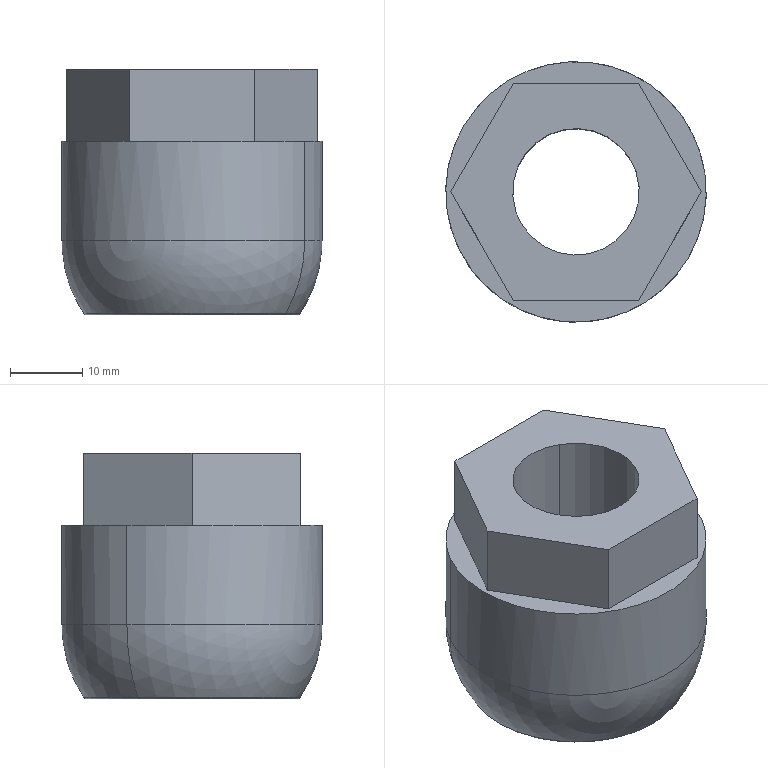NC program | NX | posted with a generic post | part box 36 x 36 x 34 mm
Lines 1 to 932 of 2807:
N10 G17 G21 G94 G90
(ZLEVEL_PROFILE , TOOL : D6C)
N12 T06 M6
N14 G54
N16 G17 G0 G90 X-11.017 Y-16.863 S4000 M3
N18 G43 Z30. H6
N20 Z1.5
N22 G94 G1 X-11.144 Y-16.717 Z1.49 F1800.
N24 X-20.05 Y-1.292 Z0.556
N26 X-20.266 Y-0.662 Z0.521
N28 X-20.34 Y0. Z0.487
N30 X-20.266 Y0.662 Z0.452
N32 X-20.05 Y1.292 Z0.417
N34 X-15.597 Y9.005 Z-0.05
N36 X-11.267 Y16.505
N38 G2 X-8.66 Y18.01 R3.01
N40 G1 X8.66
N42 G2 X11.267 Y16.505 R3.01
N44 G1 X19.927 Y1.505
N46 G2 X19.927 Y-1.505 R3.01
N48 G1 X11.267 Y-16.505
N50 G2 X8.66 Y-18.01 R3.01
N52 G1 X-8.66
N54 G2 X-11.267 Y-16.505 R3.01
N56 G1 X-19.927 Y-1.505
N58 G2 X-19.927 Y1.505 R3.01
N60 G1 X-15.597 Y9.005
N62 X-14.164 Y11.486 Z-0.1
N64 X-11.267 Y16.505
N66 G2 X-8.66 Y18.01 R3.01
N68 G1 X8.66
N70 G2 X11.267 Y16.505 R3.01
N72 G1 X19.927 Y1.505
N74 G2 X19.927 Y-1.505 R3.01
N76 G1 X11.267 Y-16.505
N78 G2 X8.66 Y-18.01 R3.01
N80 G1 X-8.66
N82 G2 X-11.267 Y-16.505 R3.01
N84 G1 X-19.927 Y-1.505
N86 G2 X-19.927 Y1.505 R3.01
N88 G1 X-15.597 Y9.005
N90 X-14.164 Y11.486 Z-0.15
N92 X-11.267 Y16.505
N94 G2 X-8.66 Y18.01 R3.01
N96 G1 X8.66
N98 G2 X11.267 Y16.505 R3.01
N100 G1 X19.927 Y1.505
N102 G2 X19.927 Y-1.505 R3.01
N104 G1 X11.267 Y-16.505
N106 G2 X8.66 Y-18.01 R3.01
N108 G1 X-8.66
N110 G2 X-11.267 Y-16.505 R3.01
N112 G1 X-19.927 Y-1.505
N114 G2 X-19.927 Y1.505 R3.01
N116 G1 X-15.597 Y9.005
N118 X-14.164 Y11.486 Z-0.2
N120 X-11.267 Y16.505
N122 G2 X-8.66 Y18.01 R3.01
N124 G1 X8.66
N126 G2 X11.267 Y16.505 R3.01
N128 G1 X19.927 Y1.505
N130 G2 X19.927 Y-1.505 R3.01
N132 G1 X11.267 Y-16.505
N134 G2 X8.66 Y-18.01 R3.01
N136 G1 X-8.66
N138 G2 X-11.267 Y-16.505 R3.01
N140 G1 X-19.927 Y-1.505
N142 G2 X-19.927 Y1.505 R3.01
N144 G1 X-15.597 Y9.005
N146 X-14.164 Y11.486 Z-0.25
N148 X-11.267 Y16.505
N150 G2 X-8.66 Y18.01 R3.01
N152 G1 X8.66
N154 G2 X11.267 Y16.505 R3.01
N156 G1 X19.927 Y1.505
N158 G2 X19.927 Y-1.505 R3.01
N160 G1 X11.267 Y-16.505
N162 G2 X8.66 Y-18.01 R3.01
N164 G1 X-8.66
N166 G2 X-11.267 Y-16.505 R3.01
N168 G1 X-19.927 Y-1.505
N170 G2 X-19.927 Y1.505 R3.01
N172 G1 X-15.597 Y9.005
N174 X-14.164 Y11.486 Z-0.3
N176 X-11.267 Y16.505
N178 G2 X-8.66 Y18.01 R3.01
N180 G1 X8.66
N182 G2 X11.267 Y16.505 R3.01
N184 G1 X19.927 Y1.505
N186 G2 X19.927 Y-1.505 R3.01
N188 G1 X11.267 Y-16.505
N190 G2 X8.66 Y-18.01 R3.01
N192 G1 X-8.66
N194 G2 X-11.267 Y-16.505 R3.01
N196 G1 X-19.927 Y-1.505
N198 G2 X-19.927 Y1.505 R3.01
N200 G1 X-15.597 Y9.005
N202 X-14.164 Y11.486 Z-0.35
N204 X-11.267 Y16.505
N206 G2 X-8.66 Y18.01 R3.01
N208 G1 X8.66
N210 G2 X11.267 Y16.505 R3.01
N212 G1 X19.927 Y1.505
N214 G2 X19.927 Y-1.505 R3.01
N216 G1 X11.267 Y-16.505
N218 G2 X8.66 Y-18.01 R3.01
N220 G1 X-8.66
N222 G2 X-11.267 Y-16.505 R3.01
N224 G1 X-19.927 Y-1.505
N226 G2 X-19.927 Y1.505 R3.01
N228 G1 X-15.597 Y9.005
N230 X-14.164 Y11.486 Z-0.4
N232 X-11.267 Y16.505
N234 G2 X-8.66 Y18.01 R3.01
N236 G1 X8.66
N238 G2 X11.267 Y16.505 R3.01
N240 G1 X19.927 Y1.505
N242 G2 X19.927 Y-1.505 R3.01
N244 G1 X11.267 Y-16.505
N246 G2 X8.66 Y-18.01 R3.01
N248 G1 X-8.66
N250 G2 X-11.267 Y-16.505 R3.01
N252 G1 X-19.927 Y-1.505
N254 G2 X-19.927 Y1.505 R3.01
N256 G1 X-15.597 Y9.005
N258 X-14.164 Y11.486 Z-0.45
N260 X-11.267 Y16.505
N262 G2 X-8.66 Y18.01 R3.01
N264 G1 X8.66
N266 G2 X11.267 Y16.505 R3.01
N268 G1 X19.927 Y1.505
N270 G2 X19.927 Y-1.505 R3.01
N272 G1 X11.267 Y-16.505
N274 G2 X8.66 Y-18.01 R3.01
N276 G1 X-8.66
N278 G2 X-11.267 Y-16.505 R3.01
N280 G1 X-19.927 Y-1.505
N282 G2 X-19.927 Y1.505 R3.01
N284 G1 X-15.597 Y9.005
N286 X-14.164 Y11.486 Z-0.5
N288 X-11.267 Y16.505
N290 G2 X-8.66 Y18.01 R3.01
N292 G1 X8.66
N294 G2 X11.267 Y16.505 R3.01
N296 G1 X19.927 Y1.505
N298 G2 X19.927 Y-1.505 R3.01
N300 G1 X11.267 Y-16.505
N302 G2 X8.66 Y-18.01 R3.01
N304 G1 X-8.66
N306 G2 X-11.267 Y-16.505 R3.01
N308 G1 X-19.927 Y-1.505
N310 G2 X-19.927 Y1.505 R3.01
N312 G1 X-15.597 Y9.005
N314 X-14.164 Y11.486 Z-0.55
N316 X-11.267 Y16.505
N318 G2 X-8.66 Y18.01 R3.01
N320 G1 X8.66
N322 G2 X11.267 Y16.505 R3.01
N324 G1 X19.927 Y1.505
N326 G2 X19.927 Y-1.505 R3.01
N328 G1 X11.267 Y-16.505
N330 G2 X8.66 Y-18.01 R3.01
N332 G1 X-8.66
N334 G2 X-11.267 Y-16.505 R3.01
N336 G1 X-19.927 Y-1.505
N338 G2 X-19.927 Y1.505 R3.01
N340 G1 X-15.597 Y9.005
N342 X-14.164 Y11.486 Z-0.6
N344 X-11.267 Y16.505
N346 G2 X-8.66 Y18.01 R3.01
N348 G1 X8.66
N350 G2 X11.267 Y16.505 R3.01
N352 G1 X19.927 Y1.505
N354 G2 X19.927 Y-1.505 R3.01
N356 G1 X11.267 Y-16.505
N358 G2 X8.66 Y-18.01 R3.01
N360 G1 X-8.66
N362 G2 X-11.267 Y-16.505 R3.01
N364 G1 X-19.927 Y-1.505
N366 G2 X-19.927 Y1.505 R3.01
N368 G1 X-15.597 Y9.005
N370 X-14.164 Y11.486 Z-0.65
N372 X-11.267 Y16.505
N374 G2 X-8.66 Y18.01 R3.01
N376 G1 X8.66
N378 G2 X11.267 Y16.505 R3.01
N380 G1 X19.927 Y1.505
N382 G2 X19.927 Y-1.505 R3.01
N384 G1 X11.267 Y-16.505
N386 G2 X8.66 Y-18.01 R3.01
N388 G1 X-8.66
N390 G2 X-11.267 Y-16.505 R3.01
N392 G1 X-19.927 Y-1.505
N394 G2 X-19.927 Y1.505 R3.01
N396 G1 X-15.597 Y9.005
N398 X-14.164 Y11.486 Z-0.7
N400 X-11.267 Y16.505
N402 G2 X-8.66 Y18.01 R3.01
N404 G1 X8.66
N406 G2 X11.267 Y16.505 R3.01
N408 G1 X19.927 Y1.505
N410 G2 X19.927 Y-1.505 R3.01
N412 G1 X11.267 Y-16.505
N414 G2 X8.66 Y-18.01 R3.01
N416 G1 X-8.66
N418 G2 X-11.267 Y-16.505 R3.01
N420 G1 X-19.927 Y-1.505
N422 G2 X-19.927 Y1.505 R3.01
N424 G1 X-15.597 Y9.005
N426 X-14.164 Y11.486 Z-0.75
N428 X-11.267 Y16.505
N430 G2 X-8.66 Y18.01 R3.01
N432 G1 X8.66
N434 G2 X11.267 Y16.505 R3.01
N436 G1 X19.927 Y1.505
N438 G2 X19.927 Y-1.505 R3.01
N440 G1 X11.267 Y-16.505
N442 G2 X8.66 Y-18.01 R3.01
N444 G1 X-8.66
N446 G2 X-11.267 Y-16.505 R3.01
N448 G1 X-19.927 Y-1.505
N450 G2 X-19.927 Y1.505 R3.01
N452 G1 X-15.597 Y9.005
N454 X-14.164 Y11.486 Z-0.8
N456 X-11.267 Y16.505
N458 G2 X-8.66 Y18.01 R3.01
N460 G1 X8.66
N462 G2 X11.267 Y16.505 R3.01
N464 G1 X19.927 Y1.505
N466 G2 X19.927 Y-1.505 R3.01
N468 G1 X11.267 Y-16.505
N470 G2 X8.66 Y-18.01 R3.01
N472 G1 X-8.66
N474 G2 X-11.267 Y-16.505 R3.01
N476 G1 X-19.927 Y-1.505
N478 G2 X-19.927 Y1.505 R3.01
N480 G1 X-15.597 Y9.005
N482 X-14.164 Y11.486 Z-0.85
N484 X-11.267 Y16.505
N486 G2 X-8.66 Y18.01 R3.01
N488 G1 X8.66
N490 G2 X11.267 Y16.505 R3.01
N492 G1 X19.927 Y1.505
N494 G2 X19.927 Y-1.505 R3.01
N496 G1 X11.267 Y-16.505
N498 G2 X8.66 Y-18.01 R3.01
N500 G1 X-8.66
N502 G2 X-11.267 Y-16.505 R3.01
N504 G1 X-19.927 Y-1.505
N506 G2 X-19.927 Y1.505 R3.01
N508 G1 X-15.597 Y9.005
N510 X-14.164 Y11.486 Z-0.9
N512 X-11.267 Y16.505
N514 G2 X-8.66 Y18.01 R3.01
N516 G1 X8.66
N518 G2 X11.267 Y16.505 R3.01
N520 G1 X19.927 Y1.505
N522 G2 X19.927 Y-1.505 R3.01
N524 G1 X11.267 Y-16.505
N526 G2 X8.66 Y-18.01 R3.01
N528 G1 X-8.66
N530 G2 X-11.267 Y-16.505 R3.01
N532 G1 X-19.927 Y-1.505
N534 G2 X-19.927 Y1.505 R3.01
N536 G1 X-15.597 Y9.005
N538 X-14.164 Y11.486 Z-0.95
N540 X-11.267 Y16.505
N542 G2 X-8.66 Y18.01 R3.01
N544 G1 X8.66
N546 G2 X11.267 Y16.505 R3.01
N548 G1 X19.927 Y1.505
N550 G2 X19.927 Y-1.505 R3.01
N552 G1 X11.267 Y-16.505
N554 G2 X8.66 Y-18.01 R3.01
N556 G1 X-8.66
N558 G2 X-11.267 Y-16.505 R3.01
N560 G1 X-19.927 Y-1.505
N562 G2 X-19.927 Y1.505 R3.01
N564 G1 X-15.597 Y9.005
N566 X-14.164 Y11.486 Z-1.
N568 X-11.267 Y16.505
N570 G2 X-8.66 Y18.01 R3.01
N572 G1 X8.66
N574 G2 X11.267 Y16.505 R3.01
N576 G1 X19.927 Y1.505
N578 G2 X19.927 Y-1.505 R3.01
N580 G1 X11.267 Y-16.505
N582 G2 X8.66 Y-18.01 R3.01
N584 G1 X-8.66
N586 G2 X-11.267 Y-16.505 R3.01
N588 G1 X-19.927 Y-1.505
N590 G2 X-19.927 Y1.505 R3.01
N592 G1 X-15.597 Y9.005
N594 X-14.164 Y11.486 Z-1.05
N596 X-11.267 Y16.505
N598 G2 X-8.66 Y18.01 R3.01
N600 G1 X8.66
N602 G2 X11.267 Y16.505 R3.01
N604 G1 X19.927 Y1.505
N606 G2 X19.927 Y-1.505 R3.01
N608 G1 X11.267 Y-16.505
N610 G2 X8.66 Y-18.01 R3.01
N612 G1 X-8.66
N614 G2 X-11.267 Y-16.505 R3.01
N616 G1 X-19.927 Y-1.505
N618 G2 X-19.927 Y1.505 R3.01
N620 G1 X-15.597 Y9.005
N622 X-14.164 Y11.486 Z-1.1
N624 X-11.267 Y16.505
N626 G2 X-8.66 Y18.01 R3.01
N628 G1 X8.66
N630 G2 X11.267 Y16.505 R3.01
N632 G1 X19.927 Y1.505
N634 G2 X19.927 Y-1.505 R3.01
N636 G1 X11.267 Y-16.505
N638 G2 X8.66 Y-18.01 R3.01
N640 G1 X-8.66
N642 G2 X-11.267 Y-16.505 R3.01
N644 G1 X-19.927 Y-1.505
N646 G2 X-19.927 Y1.505 R3.01
N648 G1 X-15.597 Y9.005
N650 X-14.164 Y11.486 Z-1.15
N652 X-11.267 Y16.505
N654 G2 X-8.66 Y18.01 R3.01
N656 G1 X8.66
N658 G2 X11.267 Y16.505 R3.01
N660 G1 X19.927 Y1.505
N662 G2 X19.927 Y-1.505 R3.01
N664 G1 X11.267 Y-16.505
N666 G2 X8.66 Y-18.01 R3.01
N668 G1 X-8.66
N670 G2 X-11.267 Y-16.505 R3.01
N672 G1 X-19.927 Y-1.505
N674 G2 X-19.927 Y1.505 R3.01
N676 G1 X-15.597 Y9.005
N678 X-14.164 Y11.486 Z-1.2
N680 X-11.267 Y16.505
N682 G2 X-8.66 Y18.01 R3.01
N684 G1 X8.66
N686 G2 X11.267 Y16.505 R3.01
N688 G1 X19.927 Y1.505
N690 G2 X19.927 Y-1.505 R3.01
N692 G1 X11.267 Y-16.505
N694 G2 X8.66 Y-18.01 R3.01
N696 G1 X-8.66
N698 G2 X-11.267 Y-16.505 R3.01
N700 G1 X-19.927 Y-1.505
N702 G2 X-19.927 Y1.505 R3.01
N704 G1 X-15.597 Y9.005
N706 X-14.164 Y11.486 Z-1.25
N708 X-11.267 Y16.505
N710 G2 X-8.66 Y18.01 R3.01
N712 G1 X8.66
N714 G2 X11.267 Y16.505 R3.01
N716 G1 X19.927 Y1.505
N718 G2 X19.927 Y-1.505 R3.01
N720 G1 X11.267 Y-16.505
N722 G2 X8.66 Y-18.01 R3.01
N724 G1 X-8.66
N726 G2 X-11.267 Y-16.505 R3.01
N728 G1 X-19.927 Y-1.505
N730 G2 X-19.927 Y1.505 R3.01
N732 G1 X-15.597 Y9.005
N734 X-14.164 Y11.486 Z-1.3
N736 X-11.267 Y16.505
N738 G2 X-8.66 Y18.01 R3.01
N740 G1 X8.66
N742 G2 X11.267 Y16.505 R3.01
N744 G1 X19.927 Y1.505
N746 G2 X19.927 Y-1.505 R3.01
N748 G1 X11.267 Y-16.505
N750 G2 X8.66 Y-18.01 R3.01
N752 G1 X-8.66
N754 G2 X-11.267 Y-16.505 R3.01
N756 G1 X-19.927 Y-1.505
N758 G2 X-19.927 Y1.505 R3.01
N760 G1 X-15.597 Y9.005
N762 X-14.164 Y11.486 Z-1.35
N764 X-11.267 Y16.505
N766 G2 X-8.66 Y18.01 R3.01
N768 G1 X8.66
N770 G2 X11.267 Y16.505 R3.01
N772 G1 X19.927 Y1.505
N774 G2 X19.927 Y-1.505 R3.01
N776 G1 X11.267 Y-16.505
N778 G2 X8.66 Y-18.01 R3.01
N780 G1 X-8.66
N782 G2 X-11.267 Y-16.505 R3.01
N784 G1 X-19.927 Y-1.505
N786 G2 X-19.927 Y1.505 R3.01
N788 G1 X-15.597 Y9.005
N790 X-14.164 Y11.486 Z-1.4
N792 X-11.267 Y16.505
N794 G2 X-8.66 Y18.01 R3.01
N796 G1 X8.66
N798 G2 X11.267 Y16.505 R3.01
N800 G1 X19.927 Y1.505
N802 G2 X19.927 Y-1.505 R3.01
N804 G1 X11.267 Y-16.505
N806 G2 X8.66 Y-18.01 R3.01
N808 G1 X-8.66
N810 G2 X-11.267 Y-16.505 R3.01
N812 G1 X-19.927 Y-1.505
N814 G2 X-19.927 Y1.505 R3.01
N816 G1 X-15.597 Y9.005
N818 X-14.164 Y11.486 Z-1.45
N820 X-11.267 Y16.505
N822 G2 X-8.66 Y18.01 R3.01
N824 G1 X8.66
N826 G2 X11.267 Y16.505 R3.01
N828 G1 X19.927 Y1.505
N830 G2 X19.927 Y-1.505 R3.01
N832 G1 X11.267 Y-16.505
N834 G2 X8.66 Y-18.01 R3.01
N836 G1 X-8.66
N838 G2 X-11.267 Y-16.505 R3.01
N840 G1 X-19.927 Y-1.505
N842 G2 X-19.927 Y1.505 R3.01
N844 G1 X-15.597 Y9.005
N846 X-14.164 Y11.486 Z-1.5
N848 X-11.267 Y16.505
N850 G2 X-8.66 Y18.01 R3.01
N852 G1 X8.66
N854 G2 X11.267 Y16.505 R3.01
N856 G1 X19.927 Y1.505
N858 G2 X19.927 Y-1.505 R3.01
N860 G1 X11.267 Y-16.505
N862 G2 X8.66 Y-18.01 R3.01
N864 G1 X-8.66
N866 G2 X-11.267 Y-16.505 R3.01
N868 G1 X-19.927 Y-1.505
N870 G2 X-19.927 Y1.505 R3.01
N872 G1 X-15.597 Y9.005
N874 X-14.164 Y11.486 Z-1.55
N876 X-11.267 Y16.505
N878 G2 X-8.66 Y18.01 R3.01
N880 G1 X8.66
N882 G2 X11.267 Y16.505 R3.01
N884 G1 X19.927 Y1.505
N886 G2 X19.927 Y-1.505 R3.01
N888 G1 X11.267 Y-16.505
N890 G2 X8.66 Y-18.01 R3.01
N892 G1 X-8.66
N894 G2 X-11.267 Y-16.505 R3.01
N896 G1 X-19.927 Y-1.505
N898 G2 X-19.927 Y1.505 R3.01
N900 G1 X-15.597 Y9.005
N902 X-14.164 Y11.486 Z-1.6
N904 X-11.267 Y16.505
N906 G2 X-8.66 Y18.01 R3.01
N908 G1 X8.66
N910 G2 X11.267 Y16.505 R3.01
N912 G1 X19.927 Y1.505
N914 G2 X19.927 Y-1.505 R3.01
N916 G1 X11.267 Y-16.505
N918 G2 X8.66 Y-18.01 R3.01
N920 G1 X-8.66
N922 G2 X-11.267 Y-16.505 R3.01
N924 G1 X-19.927 Y-1.505
N926 G2 X-19.927 Y1.505 R3.01
N928 G1 X-15.597 Y9.005
N930 X-14.164 Y11.486 Z-1.65
N932 X-11.267 Y16.505
N934 G2 X-8.66 Y18.01 R3.01
N936 G1 X8.66
N938 G2 X11.267 Y16.505 R3.01
N940 G1 X19.927 Y1.505
N942 G2 X19.927 Y-1.505 R3.01
N944 G1 X11.267 Y-16.505
N946 G2 X8.66 Y-18.01 R3.01
N948 G1 X-8.66
N950 G2 X-11.267 Y-16.505 R3.01
N952 G1 X-19.927 Y-1.505
N954 G2 X-19.927 Y1.505 R3.01
N956 G1 X-15.597 Y9.005
N958 X-14.164 Y11.486 Z-1.7
N960 X-11.267 Y16.505
N962 G2 X-8.66 Y18.01 R3.01
N964 G1 X8.66
N966 G2 X11.267 Y16.505 R3.01
N968 G1 X19.927 Y1.505
N970 G2 X19.927 Y-1.505 R3.01
N972 G1 X11.267 Y-16.505
N974 G2 X8.66 Y-18.01 R3.01
N976 G1 X-8.66
N978 G2 X-11.267 Y-16.505 R3.01
N980 G1 X-19.927 Y-1.505
N982 G2 X-19.927 Y1.505 R3.01
N984 G1 X-15.597 Y9.005
N986 X-14.164 Y11.486 Z-1.75
N988 X-11.267 Y16.505
N990 G2 X-8.66 Y18.01 R3.01
N992 G1 X8.66
N994 G2 X11.267 Y16.505 R3.01
N996 G1 X19.927 Y1.505
N998 G2 X19.927 Y-1.505 R3.01
N1000 G1 X11.267 Y-16.505
N1002 G2 X8.66 Y-18.01 R3.01
N1004 G1 X-8.66
N1006 G2 X-11.267 Y-16.505 R3.01
N1008 G1 X-19.927 Y-1.505
N1010 G2 X-19.927 Y1.505 R3.01
N1012 G1 X-15.597 Y9.005
N1014 X-14.164 Y11.486 Z-1.8
N1016 X-11.267 Y16.505
N1018 G2 X-8.66 Y18.01 R3.01
N1020 G1 X8.66
N1022 G2 X11.267 Y16.505 R3.01
N1024 G1 X19.927 Y1.505
N1026 G2 X19.927 Y-1.505 R3.01
N1028 G1 X11.267 Y-16.505
N1030 G2 X8.66 Y-18.01 R3.01
N1032 G1 X-8.66
N1034 G2 X-11.267 Y-16.505 R3.01
N1036 G1 X-19.927 Y-1.505
N1038 G2 X-19.927 Y1.505 R3.01
N1040 G1 X-15.597 Y9.005
N1042 X-14.164 Y11.486 Z-1.85
N1044 X-11.267 Y16.505
N1046 G2 X-8.66 Y18.01 R3.01
N1048 G1 X8.66
N1050 G2 X11.267 Y16.505 R3.01
N1052 G1 X19.927 Y1.505
N1054 G2 X19.927 Y-1.505 R3.01
N1056 G1 X11.267 Y-16.505
N1058 G2 X8.66 Y-18.01 R3.01
N1060 G1 X-8.66
N1062 G2 X-11.267 Y-16.505 R3.01
N1064 G1 X-19.927 Y-1.505
N1066 G2 X-19.927 Y1.505 R3.01
N1068 G1 X-15.597 Y9.005
N1070 X-14.164 Y11.486 Z-1.9
N1072 X-11.267 Y16.505
N1074 G2 X-8.66 Y18.01 R3.01
N1076 G1 X8.66
N1078 G2 X11.267 Y16.505 R3.01
N1080 G1 X19.927 Y1.505
N1082 G2 X19.927 Y-1.505 R3.01
N1084 G1 X11.267 Y-16.505
N1086 G2 X8.66 Y-18.01 R3.01
N1088 G1 X-8.66
N1090 G2 X-11.267 Y-16.505 R3.01
N1092 G1 X-19.927 Y-1.505
N1094 G2 X-19.927 Y1.505 R3.01
N1096 G1 X-15.597 Y9.005
N1098 X-14.164 Y11.486 Z-1.95
N1100 X-11.267 Y16.505
N1102 G2 X-8.66 Y18.01 R3.01
N1104 G1 X8.66
N1106 G2 X11.267 Y16.505 R3.01
N1108 G1 X19.927 Y1.505
N1110 G2 X19.927 Y-1.505 R3.01
N1112 G1 X11.267 Y-16.505
N1114 G2 X8.66 Y-18.01 R3.01
N1116 G1 X-8.66
N1118 G2 X-11.267 Y-16.505 R3.01
N1120 G1 X-19.927 Y-1.505
N1122 G2 X-19.927 Y1.505 R3.01
N1124 G1 X-15.597 Y9.005
N1126 X-14.164 Y11.486 Z-2.
N1128 X-11.267 Y16.505
N1130 G2 X-8.66 Y18.01 R3.01
N1132 G1 X8.66
N1134 G2 X11.267 Y16.505 R3.01
N1136 G1 X19.927 Y1.505
N1138 G2 X19.927 Y-1.505 R3.01
N1140 G1 X11.267 Y-16.505
N1142 G2 X8.66 Y-18.01 R3.01
N1144 G1 X-8.66
N1146 G2 X-11.267 Y-16.505 R3.01
N1148 G1 X-19.927 Y-1.505
N1150 G2 X-19.927 Y1.505 R3.01
N1152 G1 X-15.597 Y9.005
N1154 X-14.164 Y11.486 Z-2.05
N1156 X-11.267 Y16.505
N1158 G2 X-8.66 Y18.01 R3.01
N1160 G1 X8.66
N1162 G2 X11.267 Y16.505 R3.01
N1164 G1 X19.927 Y1.505
N1166 G2 X19.927 Y-1.505 R3.01
N1168 G1 X11.267 Y-16.505
N1170 G2 X8.66 Y-18.01 R3.01
N1172 G1 X-8.66
N1174 G2 X-11.267 Y-16.505 R3.01
N1176 G1 X-19.927 Y-1.505
N1178 G2 X-19.927 Y1.505 R3.01
N1180 G1 X-15.597 Y9.005
N1182 X-14.164 Y11.486 Z-2.1
N1184 X-11.267 Y16.505
N1186 G2 X-8.66 Y18.01 R3.01
N1188 G1 X8.66
N1190 G2 X11.267 Y16.505 R3.01
N1192 G1 X19.927 Y1.505
N1194 G2 X19.927 Y-1.505 R3.01
N1196 G1 X11.267 Y-16.505
N1198 G2 X8.66 Y-18.01 R3.01
N1200 G1 X-8.66
N1202 G2 X-11.267 Y-16.505 R3.01
N1204 G1 X-19.927 Y-1.505
N1206 G2 X-19.927 Y1.505 R3.01
N1208 G1 X-15.597 Y9.005
N1210 X-14.164 Y11.486 Z-2.15
N1212 X-11.267 Y16.505
N1214 G2 X-8.66 Y18.01 R3.01
N1216 G1 X8.66
N1218 G2 X11.267 Y16.505 R3.01
N1220 G1 X19.927 Y1.505
N1222 G2 X19.927 Y-1.505 R3.01
N1224 G1 X11.267 Y-16.505
N1226 G2 X8.66 Y-18.01 R3.01
N1228 G1 X-8.66
N1230 G2 X-11.267 Y-16.505 R3.01
N1232 G1 X-19.927 Y-1.505
N1234 G2 X-19.927 Y1.505 R3.01
N1236 G1 X-15.597 Y9.005
N1238 X-14.164 Y11.486 Z-2.2
N1240 X-11.267 Y16.505
N1242 G2 X-8.66 Y18.01 R3.01
N1244 G1 X8.66
N1246 G2 X11.267 Y16.505 R3.01
N1248 G1 X19.927 Y1.505
N1250 G2 X19.927 Y-1.505 R3.01
N1252 G1 X11.267 Y-16.505
N1254 G2 X8.66 Y-18.01 R3.01
N1256 G1 X-8.66
N1258 G2 X-11.267 Y-16.505 R3.01
N1260 G1 X-19.927 Y-1.505
N1262 G2 X-19.927 Y1.505 R3.01
N1264 G1 X-15.597 Y9.005
N1266 X-14.164 Y11.486 Z-2.25
N1268 X-11.267 Y16.505
N1270 G2 X-8.66 Y18.01 R3.01
N1272 G1 X8.66
N1274 G2 X11.267 Y16.505 R3.01
N1276 G1 X19.927 Y1.505
N1278 G2 X19.927 Y-1.505 R3.01
N1280 G1 X11.267 Y-16.505
N1282 G2 X8.66 Y-18.01 R3.01
N1284 G1 X-8.66
N1286 G2 X-11.267 Y-16.505 R3.01
N1288 G1 X-19.927 Y-1.505
N1290 G2 X-19.927 Y1.505 R3.01
N1292 G1 X-15.597 Y9.005
N1294 X-14.164 Y11.486 Z-2.3
N1296 X-11.267 Y16.505
N1298 G2 X-8.66 Y18.01 R3.01
N1300 G1 X8.66
N1302 G2 X11.267 Y16.505 R3.01
N1304 G1 X19.927 Y1.505
N1306 G2 X19.927 Y-1.505 R3.01
N1308 G1 X11.267 Y-16.505
N1310 G2 X8.66 Y-18.01 R3.01
N1312 G1 X-8.66
N1314 G2 X-11.267 Y-16.505 R3.01
N1316 G1 X-19.927 Y-1.505
N1318 G2 X-19.927 Y1.505 R3.01
N1320 G1 X-15.597 Y9.005
N1322 X-14.164 Y11.486 Z-2.35
N1324 X-11.267 Y16.505
N1326 G2 X-8.66 Y18.01 R3.01
N1328 G1 X8.66
N1330 G2 X11.267 Y16.505 R3.01
N1332 G1 X19.927 Y1.505
N1334 G2 X19.927 Y-1.505 R3.01
N1336 G1 X11.267 Y-16.505
N1338 G2 X8.66 Y-18.01 R3.01
N1340 G1 X-8.66
N1342 G2 X-11.267 Y-16.505 R3.01
N1344 G1 X-19.927 Y-1.505
N1346 G2 X-19.927 Y1.505 R3.01
N1348 G1 X-15.597 Y9.005
N1350 X-14.164 Y11.486 Z-2.4
N1352 X-11.267 Y16.505
N1354 G2 X-8.66 Y18.01 R3.01
N1356 G1 X8.66
N1358 G2 X11.267 Y16.505 R3.01
N1360 G1 X19.927 Y1.505
N1362 G2 X19.927 Y-1.505 R3.01
N1364 G1 X11.267 Y-16.505
N1366 G2 X8.66 Y-18.01 R3.01
N1368 G1 X-8.66
N1370 G2 X-11.267 Y-16.505 R3.01
N1372 G1 X-19.927 Y-1.505
N1374 G2 X-19.927 Y1.505 R3.01
N1376 G1 X-15.597 Y9.005
N1378 X-14.164 Y11.486 Z-2.45
N1380 X-11.267 Y16.505
N1382 G2 X-8.66 Y18.01 R3.01
N1384 G1 X8.66
N1386 G2 X11.267 Y16.505 R3.01
N1388 G1 X19.927 Y1.505
N1390 G2 X19.927 Y-1.505 R3.01
N1392 G1 X11.267 Y-16.505
N1394 G2 X8.66 Y-18.01 R3.01
N1396 G1 X-8.66
N1398 G2 X-11.267 Y-16.505 R3.01
N1400 G1 X-19.927 Y-1.505
N1402 G2 X-19.927 Y1.505 R3.01
N1404 G1 X-15.597 Y9.005
N1406 X-14.164 Y11.486 Z-2.5
N1408 X-11.267 Y16.505
N1410 G2 X-8.66 Y18.01 R3.01
N1412 G1 X8.66
N1414 G2 X11.267 Y16.505 R3.01
N1416 G1 X19.927 Y1.505
N1418 G2 X19.927 Y-1.505 R3.01
N1420 G1 X11.267 Y-16.505
N1422 G2 X8.66 Y-18.01 R3.01
N1424 G1 X-8.66
N1426 G2 X-11.267 Y-16.505 R3.01
N1428 G1 X-19.927 Y-1.505
N1430 G2 X-19.927 Y1.505 R3.01
N1432 G1 X-15.597 Y9.005
N1434 X-14.164 Y11.486 Z-2.55
N1436 X-11.267 Y16.505
N1438 G2 X-8.66 Y18.01 R3.01
N1440 G1 X8.66
N1442 G2 X11.267 Y16.505 R3.01
N1444 G1 X19.927 Y1.505
N1446 G2 X19.927 Y-1.505 R3.01
N1448 G1 X11.267 Y-16.505
N1450 G2 X8.66 Y-18.01 R3.01
N1452 G1 X-8.66
N1454 G2 X-11.267 Y-16.505 R3.01
N1456 G1 X-19.927 Y-1.505
N1458 G2 X-19.927 Y1.505 R3.01
N1460 G1 X-15.597 Y9.005
N1462 X-14.164 Y11.486 Z-2.6
N1464 X-11.267 Y16.505
N1466 G2 X-8.66 Y18.01 R3.01
N1468 G1 X8.66
N1470 G2 X11.267 Y16.505 R3.01
N1472 G1 X19.927 Y1.505
N1474 G2 X19.927 Y-1.505 R3.01
N1476 G1 X11.267 Y-16.505
N1478 G2 X8.66 Y-18.01 R3.01
N1480 G1 X-8.66
N1482 G2 X-11.267 Y-16.505 R3.01
N1484 G1 X-19.927 Y-1.505
N1486 G2 X-19.927 Y1.505 R3.01
N1488 G1 X-15.597 Y9.005
N1490 X-14.164 Y11.486 Z-2.65
N1492 X-11.267 Y16.505
N1494 G2 X-8.66 Y18.01 R3.01
N1496 G1 X8.66
N1498 G2 X11.267 Y16.505 R3.01
N1500 G1 X19.927 Y1.505
N1502 G2 X19.927 Y-1.505 R3.01
N1504 G1 X11.267 Y-16.505
N1506 G2 X8.66 Y-18.01 R3.01
N1508 G1 X-8.66
N1510 G2 X-11.267 Y-16.505 R3.01
N1512 G1 X-19.927 Y-1.505
N1514 G2 X-19.927 Y1.505 R3.01
N1516 G1 X-15.597 Y9.005
N1518 X-14.164 Y11.486 Z-2.7
N1520 X-11.267 Y16.505
N1522 G2 X-8.66 Y18.01 R3.01
N1524 G1 X8.66
N1526 G2 X11.267 Y16.505 R3.01
N1528 G1 X19.927 Y1.505
N1530 G2 X19.927 Y-1.505 R3.01
N1532 G1 X11.267 Y-16.505
N1534 G2 X8.66 Y-18.01 R3.01
N1536 G1 X-8.66
N1538 G2 X-11.267 Y-16.505 R3.01
N1540 G1 X-19.927 Y-1.505
N1542 G2 X-19.927 Y1.505 R3.01
N1544 G1 X-15.597 Y9.005
N1546 X-14.164 Y11.486 Z-2.75
N1548 X-11.267 Y16.505
N1550 G2 X-8.66 Y18.01 R3.01
N1552 G1 X8.66
N1554 G2 X11.267 Y16.505 R3.01
N1556 G1 X19.927 Y1.505
N1558 G2 X19.927 Y-1.505 R3.01
N1560 G1 X11.267 Y-16.505
N1562 G2 X8.66 Y-18.01 R3.01
N1564 G1 X-8.66
N1566 G2 X-11.267 Y-16.505 R3.01
N1568 G1 X-19.927 Y-1.505
N1570 G2 X-19.927 Y1.505 R3.01
N1572 G1 X-15.597 Y9.005
N1574 X-14.164 Y11.486 Z-2.8
N1576 X-11.267 Y16.505
N1578 G2 X-8.66 Y18.01 R3.01
N1580 G1 X8.66
N1582 G2 X11.267 Y16.505 R3.01
N1584 G1 X19.927 Y1.505
N1586 G2 X19.927 Y-1.505 R3.01
N1588 G1 X11.267 Y-16.505
N1590 G2 X8.66 Y-18.01 R3.01
N1592 G1 X-8.66
N1594 G2 X-11.267 Y-16.505 R3.01
N1596 G1 X-19.927 Y-1.505
N1598 G2 X-19.927 Y1.505 R3.01
N1600 G1 X-15.597 Y9.005
N1602 X-14.164 Y11.486 Z-2.85
N1604 X-11.267 Y16.505
N1606 G2 X-8.66 Y18.01 R3.01
N1608 G1 X8.66
N1610 G2 X11.267 Y16.505 R3.01
N1612 G1 X19.927 Y1.505
N1614 G2 X19.927 Y-1.505 R3.01
N1616 G1 X11.267 Y-16.505
N1618 G2 X8.66 Y-18.01 R3.01
N1620 G1 X-8.66
N1622 G2 X-11.267 Y-16.505 R3.01
N1624 G1 X-19.927 Y-1.505
N1626 G2 X-19.927 Y1.505 R3.01
N1628 G1 X-15.597 Y9.005
N1630 X-14.164 Y11.486 Z-2.9
N1632 X-11.267 Y16.505
N1634 G2 X-8.66 Y18.01 R3.01
N1636 G1 X8.66
N1638 G2 X11.267 Y16.505 R3.01
N1640 G1 X19.927 Y1.505
N1642 G2 X19.927 Y-1.505 R3.01
N1644 G1 X11.267 Y-16.505
N1646 G2 X8.66 Y-18.01 R3.01
N1648 G1 X-8.66
N1650 G2 X-11.267 Y-16.505 R3.01
N1652 G1 X-19.927 Y-1.505
N1654 G2 X-19.927 Y1.505 R3.01
N1656 G1 X-15.597 Y9.005
N1658 X-14.164 Y11.486 Z-2.95
N1660 X-11.267 Y16.505
N1662 G2 X-8.66 Y18.01 R3.01
N1664 G1 X8.66
N1666 G2 X11.267 Y16.505 R3.01
N1668 G1 X19.927 Y1.505
N1670 G2 X19.927 Y-1.505 R3.01
N1672 G1 X11.267 Y-16.505
N1674 G2 X8.66 Y-18.01 R3.01
N1676 G1 X-8.66
N1678 G2 X-11.267 Y-16.505 R3.01
N1680 G1 X-19.927 Y-1.505
N1682 G2 X-19.927 Y1.505 R3.01
N1684 G1 X-15.597 Y9.005
N1686 X-14.164 Y11.486 Z-3.
N1688 X-11.267 Y16.505
N1690 G2 X-8.66 Y18.01 R3.01
N1692 G1 X8.66
N1694 G2 X11.267 Y16.505 R3.01
N1696 G1 X19.927 Y1.505
N1698 G2 X19.927 Y-1.505 R3.01
N1700 G1 X11.267 Y-16.505
N1702 G2 X8.66 Y-18.01 R3.01
N1704 G1 X-8.66
N1706 G2 X-11.267 Y-16.505 R3.01
N1708 G1 X-19.927 Y-1.505
N1710 G2 X-19.927 Y1.505 R3.01
N1712 G1 X-15.597 Y9.005
N1714 X-14.164 Y11.486 Z-3.05
N1716 X-11.267 Y16.505
N1718 G2 X-8.66 Y18.01 R3.01
N1720 G1 X8.66
N1722 G2 X11.267 Y16.505 R3.01
N1724 G1 X19.927 Y1.505
N1726 G2 X19.927 Y-1.505 R3.01
N1728 G1 X11.267 Y-16.505
N1730 G2 X8.66 Y-18.01 R3.01
N1732 G1 X-8.66
N1734 G2 X-11.267 Y-16.505 R3.01
N1736 G1 X-19.927 Y-1.505
N1738 G2 X-19.927 Y1.505 R3.01
N1740 G1 X-15.597 Y9.005
N1742 X-14.164 Y11.486 Z-3.1
N1744 X-11.267 Y16.505
N1746 G2 X-8.66 Y18.01 R3.01
N1748 G1 X8.66
N1750 G2 X11.267 Y16.505 R3.01
N1752 G1 X19.927 Y1.505
N1754 G2 X19.927 Y-1.505 R3.01
N1756 G1 X11.267 Y-16.505
N1758 G2 X8.66 Y-18.01 R3.01
N1760 G1 X-8.66
N1762 G2 X-11.267 Y-16.505 R3.01
N1764 G1 X-19.927 Y-1.505
N1766 G2 X-19.927 Y1.505 R3.01
N1768 G1 X-15.597 Y9.005
N1770 X-14.164 Y11.486 Z-3.15
N1772 X-11.267 Y16.505
N1774 G2 X-8.66 Y18.01 R3.01
N1776 G1 X8.66
N1778 G2 X11.267 Y16.505 R3.01
N1780 G1 X19.927 Y1.505
N1782 G2 X19.927 Y-1.505 R3.01
N1784 G1 X11.267 Y-16.505
N1786 G2 X8.66 Y-18.01 R3.01
N1788 G1 X-8.66
N1790 G2 X-11.267 Y-16.505 R3.01
N1792 G1 X-19.927 Y-1.505
N1794 G2 X-19.927 Y1.505 R3.01
N1796 G1 X-15.597 Y9.005
N1798 X-14.164 Y11.486 Z-3.2
N1800 X-11.267 Y16.505
N1802 G2 X-8.66 Y18.01 R3.01
N1804 G1 X8.66
N1806 G2 X11.267 Y16.505 R3.01
N1808 G1 X19.927 Y1.505
N1810 G2 X19.927 Y-1.505 R3.01
N1812 G1 X11.267 Y-16.505
N1814 G2 X8.66 Y-18.01 R3.01
N1816 G1 X-8.66
N1818 G2 X-11.267 Y-16.505 R3.01
N1820 G1 X-19.927 Y-1.505
N1822 G2 X-19.927 Y1.505 R3.01
N1824 G1 X-15.597 Y9.005
N1826 X-14.164 Y11.486 Z-3.25
N1828 X-11.267 Y16.505
N1830 G2 X-8.66 Y18.01 R3.01
N1832 G1 X8.66
N1834 G2 X11.267 Y16.505 R3.01
N1836 G1 X19.927 Y1.505
N1838 G2 X19.927 Y-1.505 R3.01
N1840 G1 X11.267 Y-16.505
N1842 G2 X8.66 Y-18.01 R3.01
N1844 G1 X-8.66
N1846 G2 X-11.267 Y-16.505 R3.01
N1848 G1 X-19.927 Y-1.505
N1850 G2 X-19.927 Y1.505 R3.01
N1852 G1 X-15.597 Y9.005
N1854 X-14.164 Y11.486 Z-3.3
N1856 X-11.267 Y16.505
N1858 G2 X-8.66 Y18.01 R3.01
N1860 G1 X8.66
N1862 G2 X11.267 Y16.505 R3.01